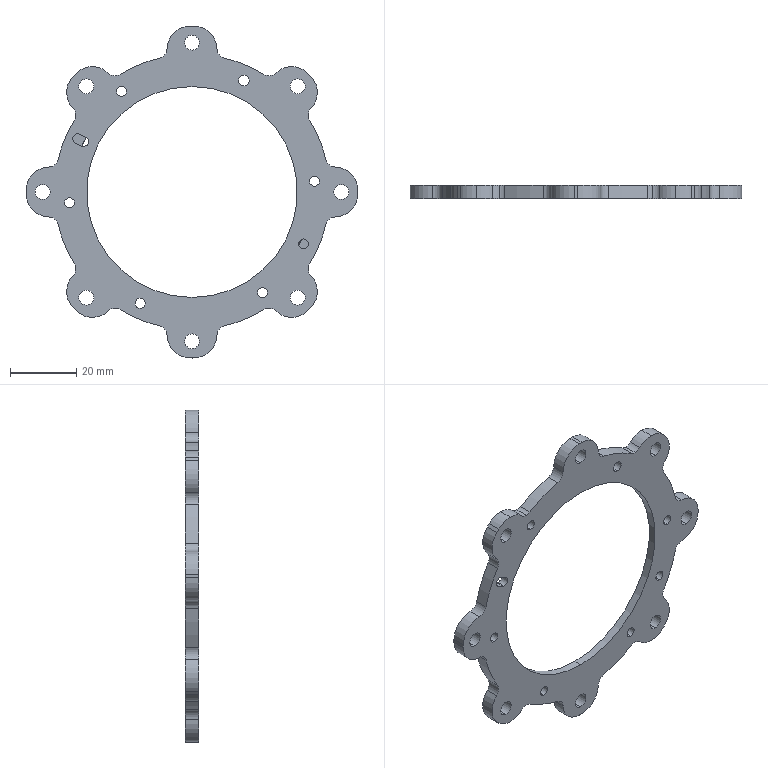Part | SolidWorks | features ICE 11, CirPattern 3, Fillet 2, Extrusion 1 | 1 solid | 115 faces | box 100 x 4 x 100 mm | volume 10292 mm3 | cylinder 108 | plane 7 | commonest cylinder face diameters 14 x19 6 x18 4.5 x16 3 x15 7 x12 100 x9